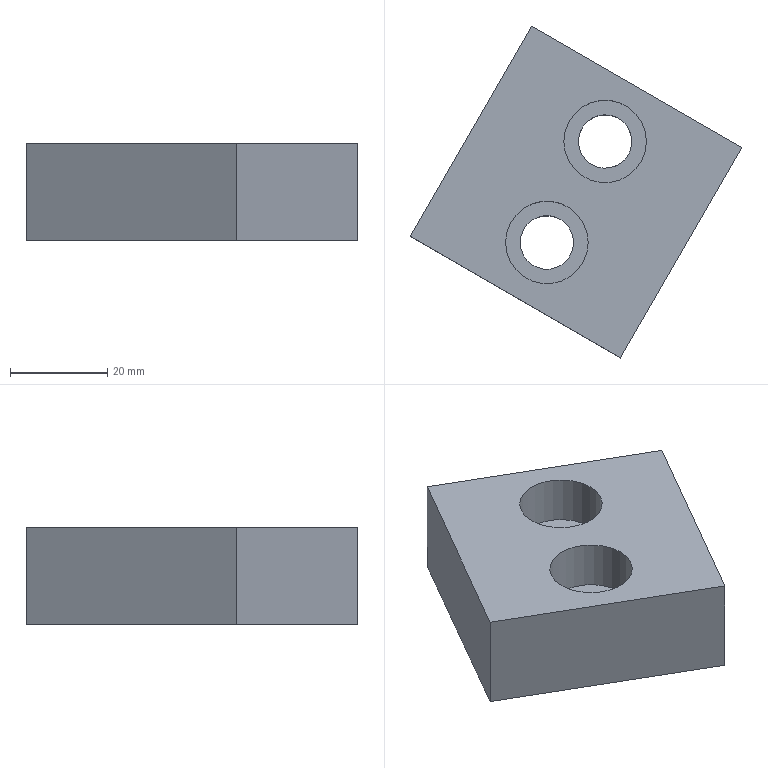Part | NX | features solid 2 | 1 solid | 12 faces | box 68.301 x 68.301 x 20 mm | volume 43560 mm3 | plane 8 | cylinder 4 | commonest cylinder face diameters 11 x2 17 x2
STEP:
#1=CARTESIAN_POINT('',(643.391,202.218,30.));
#2=VERTEX_POINT('',#1);
#3=CARTESIAN_POINT('',(668.391,245.519,30.));
#4=VERTEX_POINT('',#3);
#5=CARTESIAN_POINT('',(655.891,223.869,30.));
#6=DIRECTION('',(-0.5,-0.866,0.));
#7=VECTOR('',#6,1000.);
#8=LINE('',#5,#7);
#9=EDGE_CURVE('',#2,#4,#8,.F.);
#10=ORIENTED_EDGE('',*,*,#9,.T.);
#11=CARTESIAN_POINT('',(625.09,270.519,30.));
#12=VERTEX_POINT('',#11);
#13=CARTESIAN_POINT('',(721.058,215.112,30.));
#14=DIRECTION('',(0.866,-0.5,0.));
#15=VECTOR('',#14,1000.);
#16=LINE('',#13,#15);
#17=EDGE_CURVE('',#4,#12,#16,.F.);
#18=ORIENTED_EDGE('',*,*,#17,.T.);
#19=CARTESIAN_POINT('',(600.09,227.218,30.));
#20=VERTEX_POINT('',#19);
#21=CARTESIAN_POINT('',(625.09,270.519,30.));
#22=DIRECTION('',(0.5,0.866,0.));
#23=VECTOR('',#22,1000.);
#24=LINE('',#21,#23);
#25=EDGE_CURVE('',#12,#20,#24,.F.);
#26=ORIENTED_EDGE('',*,*,#25,.T.);
#27=CARTESIAN_POINT('',(696.058,171.811,30.));
#28=DIRECTION('',(-0.866,0.5,0.));
#29=VECTOR('',#28,1000.);
#30=LINE('',#27,#29);
#31=EDGE_CURVE('',#2,#20,#30,.T.);
#32=ORIENTED_EDGE('',*,*,#31,.F.);
#33=EDGE_LOOP('',(#10,#18,#26,#32));
#34=FACE_BOUND('',#33,.T.);
#35=CARTESIAN_POINT('',(636.74,225.976,30.));
#36=VERTEX_POINT('',#35);
#37=CARTESIAN_POINT('',(628.24,225.976,30.));
#38=DIRECTION('',(0.,0.,1.));
#39=DIRECTION('',(1.,0.,0.));
#40=AXIS2_PLACEMENT_3D('',#37,#38,#39);
#41=CIRCLE('',#40,8.5);
#42=EDGE_CURVE('',#36,#36,#41,.F.);
#43=ORIENTED_EDGE('',*,*,#42,.T.);
#44=EDGE_LOOP('',(#43));
#45=FACE_BOUND('',#44,.T.);
#46=CARTESIAN_POINT('',(648.74,246.761,30.));
#47=VERTEX_POINT('',#46);
#48=CARTESIAN_POINT('',(640.24,246.761,30.));
#49=DIRECTION('',(0.,0.,1.));
#50=DIRECTION('',(1.,0.,0.));
#51=AXIS2_PLACEMENT_3D('',#48,#49,#50);
#52=CIRCLE('',#51,8.5);
#53=EDGE_CURVE('',#47,#47,#52,.T.);
#54=ORIENTED_EDGE('',*,*,#53,.F.);
#55=EDGE_LOOP('',(#54));
#56=FACE_BOUND('',#55,.T.);
#57=CARTESIAN_POINT('',(751.058,267.073,30.));
#58=DIRECTION('',(0.,0.,1.));
#59=DIRECTION('',(-0.5,-0.866,0.));
#60=AXIS2_PLACEMENT_3D('',#57,#58,#59);
#61=PLANE('',#60);
#62=ADVANCED_FACE('',(#34,#45,#56),#61,.T.);
#63=CARTESIAN_POINT('',(622.74,225.976,10.));
#64=VERTEX_POINT('',#63);
#65=CARTESIAN_POINT('',(628.24,225.976,10.));
#66=DIRECTION('',(0.,0.,-1.));
#67=DIRECTION('',(-1.,0.,0.));
#68=AXIS2_PLACEMENT_3D('',#65,#66,#67);
#69=CIRCLE('',#68,5.5);
#70=EDGE_CURVE('',#64,#64,#69,.F.);
#71=ORIENTED_EDGE('',*,*,#70,.F.);
#72=EDGE_LOOP('',(#71));
#73=FACE_BOUND('',#72,.T.);
#74=CARTESIAN_POINT('',(622.74,225.976,20.));
#75=VERTEX_POINT('',#74);
#76=CARTESIAN_POINT('',(628.24,225.976,20.));
#77=DIRECTION('',(0.,0.,-1.));
#78=DIRECTION('',(-1.,0.,0.));
#79=AXIS2_PLACEMENT_3D('',#76,#77,#78);
#80=CIRCLE('',#79,5.5);
#81=EDGE_CURVE('',#75,#75,#80,.T.);
#82=ORIENTED_EDGE('',*,*,#81,.F.);
#83=EDGE_LOOP('',(#82));
#84=FACE_BOUND('',#83,.T.);
#85=CARTESIAN_POINT('',(628.24,225.976,30.));
#86=DIRECTION('',(0.,0.,-1.));
#87=DIRECTION('',(1.,0.,0.));
#88=AXIS2_PLACEMENT_3D('',#85,#86,#87);
#89=CYLINDRICAL_SURFACE('',#88,5.5);
#90=ADVANCED_FACE('',(#73,#84),#89,.F.);
#91=ORIENTED_EDGE('',*,*,#70,.T.);
#92=EDGE_LOOP('',(#91));
#93=FACE_BOUND('',#92,.T.);
#94=CARTESIAN_POINT('',(668.391,245.519,10.));
#95=VERTEX_POINT('',#94);
#96=CARTESIAN_POINT('',(643.391,202.218,10.));
#97=VERTEX_POINT('',#96);
#98=CARTESIAN_POINT('',(655.891,223.869,10.));
#99=DIRECTION('',(-0.5,-0.866,0.));
#100=VECTOR('',#99,1000.);
#101=LINE('',#98,#100);
#102=EDGE_CURVE('',#95,#97,#101,.T.);
#103=ORIENTED_EDGE('',*,*,#102,.T.);
#104=CARTESIAN_POINT('',(600.09,227.218,10.));
#105=VERTEX_POINT('',#104);
#106=CARTESIAN_POINT('',(696.058,171.811,10.));
#107=DIRECTION('',(0.866,-0.5,0.));
#108=VECTOR('',#107,1000.);
#109=LINE('',#106,#108);
#110=EDGE_CURVE('',#97,#105,#109,.F.);
#111=ORIENTED_EDGE('',*,*,#110,.T.);
#112=CARTESIAN_POINT('',(625.09,270.519,10.));
#113=VERTEX_POINT('',#112);
#114=CARTESIAN_POINT('',(448.115,-36.01,10.));
#115=DIRECTION('',(-0.5,-0.866,0.));
#116=VECTOR('',#115,1000.);
#117=LINE('',#114,#116);
#118=EDGE_CURVE('',#113,#105,#117,.T.);
#119=ORIENTED_EDGE('',*,*,#118,.F.);
#120=CARTESIAN_POINT('',(1116.975,-13.471,10.));
#121=DIRECTION('',(-0.866,0.5,0.));
#122=VECTOR('',#121,1000.);
#123=LINE('',#120,#122);
#124=EDGE_CURVE('',#95,#113,#123,.T.);
#125=ORIENTED_EDGE('',*,*,#124,.F.);
#126=EDGE_LOOP('',(#103,#111,#119,#125));
#127=FACE_BOUND('',#126,.T.);
#128=CARTESIAN_POINT('',(634.74,246.761,10.));
#129=VERTEX_POINT('',#128);
#130=CARTESIAN_POINT('',(640.24,246.761,10.));
#131=DIRECTION('',(0.,0.,-1.));
#132=DIRECTION('',(-1.,0.,0.));
#133=AXIS2_PLACEMENT_3D('',#130,#131,#132);
#134=CIRCLE('',#133,5.5);
#135=EDGE_CURVE('',#129,#129,#134,.F.);
#136=ORIENTED_EDGE('',*,*,#135,.T.);
#137=EDGE_LOOP('',(#136));
#138=FACE_BOUND('',#137,.T.);
#139=CARTESIAN_POINT('',(940.,-320.,10.));
#140=DIRECTION('',(0.,0.,1.));
#141=DIRECTION('',(0.,1.,0.));
#142=AXIS2_PLACEMENT_3D('',#139,#140,#141);
#143=PLANE('',#142);
#144=ADVANCED_FACE('',(#93,#127,#138),#143,.F.);
#145=CARTESIAN_POINT('',(668.391,245.519,25.));
#146=DIRECTION('',(0.,0.,-1.));
#147=VECTOR('',#146,1000.);
#148=LINE('',#145,#147);
#149=EDGE_CURVE('',#4,#95,#148,.T.);
#150=ORIENTED_EDGE('',*,*,#149,.T.);
#151=ORIENTED_EDGE('',*,*,#124,.T.);
#152=CARTESIAN_POINT('',(625.09,270.519,80.));
#153=DIRECTION('',(0.,0.,-1.));
#154=VECTOR('',#153,1000.);
#155=LINE('',#152,#154);
#156=EDGE_CURVE('',#12,#113,#155,.T.);
#157=ORIENTED_EDGE('',*,*,#156,.F.);
#158=ORIENTED_EDGE('',*,*,#17,.F.);
#159=EDGE_LOOP('',(#150,#151,#157,#158));
#160=FACE_BOUND('',#159,.T.);
#161=CARTESIAN_POINT('',(721.058,215.112,80.));
#162=DIRECTION('',(-0.5,-0.866,0.));
#163=DIRECTION('',(0.,0.,-1.));
#164=AXIS2_PLACEMENT_3D('',#161,#162,#163);
#165=PLANE('',#164);
#166=ADVANCED_FACE('',(#160),#165,.F.);
#167=CARTESIAN_POINT('',(643.391,202.218,25.));
#168=DIRECTION('',(0.,0.,-1.));
#169=VECTOR('',#168,1000.);
#170=LINE('',#167,#169);
#171=EDGE_CURVE('',#97,#2,#170,.F.);
#172=ORIENTED_EDGE('',*,*,#171,.T.);
#173=ORIENTED_EDGE('',*,*,#31,.T.);
#174=CARTESIAN_POINT('',(600.09,227.218,20.));
#175=DIRECTION('',(0.,0.,1.));
#176=VECTOR('',#175,1000.);
#177=LINE('',#174,#176);
#178=EDGE_CURVE('',#20,#105,#177,.F.);
#179=ORIENTED_EDGE('',*,*,#178,.T.);
#180=ORIENTED_EDGE('',*,*,#110,.F.);
#181=EDGE_LOOP('',(#172,#173,#179,#180));
#182=FACE_BOUND('',#181,.T.);
#183=CARTESIAN_POINT('',(696.058,171.811,80.));
#184=DIRECTION('',(-0.5,-0.866,0.));
#185=DIRECTION('',(0.,0.,-1.));
#186=AXIS2_PLACEMENT_3D('',#183,#184,#185);
#187=PLANE('',#186);
#188=ADVANCED_FACE('',(#182),#187,.T.);
#189=ORIENTED_EDGE('',*,*,#118,.T.);
#190=ORIENTED_EDGE('',*,*,#178,.F.);
#191=ORIENTED_EDGE('',*,*,#25,.F.);
#192=ORIENTED_EDGE('',*,*,#156,.T.);
#193=EDGE_LOOP('',(#189,#190,#191,#192));
#194=FACE_BOUND('',#193,.T.);
#195=CARTESIAN_POINT('',(625.09,270.519,20.));
#196=DIRECTION('',(-0.866,0.5,0.));
#197=DIRECTION('',(0.5,0.866,0.));
#198=AXIS2_PLACEMENT_3D('',#195,#196,#197);
#199=PLANE('',#198);
#200=ADVANCED_FACE('',(#194),#199,.T.);
#201=ORIENTED_EDGE('',*,*,#171,.F.);
#202=ORIENTED_EDGE('',*,*,#102,.F.);
#203=ORIENTED_EDGE('',*,*,#149,.F.);
#204=ORIENTED_EDGE('',*,*,#9,.F.);
#205=EDGE_LOOP('',(#201,#202,#203,#204));
#206=FACE_BOUND('',#205,.T.);
#207=CARTESIAN_POINT('',(655.891,223.869,25.));
#208=DIRECTION('',(0.866,-0.5,0.));
#209=DIRECTION('',(-0.5,-0.866,0.));
#210=AXIS2_PLACEMENT_3D('',#207,#208,#209);
#211=PLANE('',#210);
#212=ADVANCED_FACE('',(#206),#211,.T.);
#213=CARTESIAN_POINT('',(637.49,251.524,20.));
#214=VERTEX_POINT('',#213);
#215=CARTESIAN_POINT('',(640.24,246.761,20.));
#216=DIRECTION('',(0.,0.,1.));
#217=DIRECTION('',(-0.5,0.866,0.));
#218=AXIS2_PLACEMENT_3D('',#215,#216,#217);
#219=CIRCLE('',#218,5.5);
#220=EDGE_CURVE('',#214,#214,#219,.T.);
#221=ORIENTED_EDGE('',*,*,#220,.T.);
#222=EDGE_LOOP('',(#221));
#223=FACE_BOUND('',#222,.T.);
#224=ORIENTED_EDGE('',*,*,#135,.F.);
#225=EDGE_LOOP('',(#224));
#226=FACE_BOUND('',#225,.T.);
#227=CARTESIAN_POINT('',(640.24,246.761,30.));
#228=DIRECTION('',(0.,0.,-1.));
#229=DIRECTION('',(0.5,-0.866,0.));
#230=AXIS2_PLACEMENT_3D('',#227,#228,#229);
#231=CYLINDRICAL_SURFACE('',#230,5.5);
#232=ADVANCED_FACE('',(#223,#226),#231,.F.);
#233=CARTESIAN_POINT('',(619.74,225.976,20.));
#234=VERTEX_POINT('',#233);
#235=CARTESIAN_POINT('',(628.24,225.976,20.));
#236=DIRECTION('',(0.,0.,-1.));
#237=DIRECTION('',(-1.,0.,0.));
#238=AXIS2_PLACEMENT_3D('',#235,#236,#237);
#239=CIRCLE('',#238,8.5);
#240=EDGE_CURVE('',#234,#234,#239,.T.);
#241=ORIENTED_EDGE('',*,*,#240,.T.);
#242=EDGE_LOOP('',(#241));
#243=FACE_BOUND('',#242,.T.);
#244=ORIENTED_EDGE('',*,*,#42,.F.);
#245=EDGE_LOOP('',(#244));
#246=FACE_BOUND('',#245,.T.);
#247=CARTESIAN_POINT('',(628.24,225.976,35.));
#248=DIRECTION('',(0.,0.,-1.));
#249=DIRECTION('',(-1.,0.,0.));
#250=AXIS2_PLACEMENT_3D('',#247,#248,#249);
#251=CYLINDRICAL_SURFACE('',#250,8.5);
#252=ADVANCED_FACE('',(#243,#246),#251,.F.);
#253=ORIENTED_EDGE('',*,*,#240,.F.);
#254=EDGE_LOOP('',(#253));
#255=FACE_BOUND('',#254,.T.);
#256=ORIENTED_EDGE('',*,*,#81,.T.);
#257=EDGE_LOOP('',(#256));
#258=FACE_BOUND('',#257,.T.);
#259=CARTESIAN_POINT('',(628.946,225.569,20.));
#260=DIRECTION('',(0.,0.,1.));
#261=DIRECTION('',(1.,0.,0.));
#262=AXIS2_PLACEMENT_3D('',#259,#260,#261);
#263=PLANE('',#262);
#264=ADVANCED_FACE('',(#255,#258),#263,.T.);
#265=CARTESIAN_POINT('',(631.74,246.761,20.));
#266=VERTEX_POINT('',#265);
#267=CARTESIAN_POINT('',(640.24,246.761,20.));
#268=DIRECTION('',(0.,0.,-1.));
#269=DIRECTION('',(-1.,0.,0.));
#270=AXIS2_PLACEMENT_3D('',#267,#268,#269);
#271=CIRCLE('',#270,8.5);
#272=EDGE_CURVE('',#266,#266,#271,.F.);
#273=ORIENTED_EDGE('',*,*,#272,.F.);
#274=EDGE_LOOP('',(#273));
#275=FACE_BOUND('',#274,.T.);
#276=ORIENTED_EDGE('',*,*,#53,.T.);
#277=EDGE_LOOP('',(#276));
#278=FACE_BOUND('',#277,.T.);
#279=CARTESIAN_POINT('',(640.24,246.761,35.));
#280=DIRECTION('',(0.,0.,-1.));
#281=DIRECTION('',(-1.,0.,0.));
#282=AXIS2_PLACEMENT_3D('',#279,#280,#281);
#283=CYLINDRICAL_SURFACE('',#282,8.5);
#284=ADVANCED_FACE('',(#275,#278),#283,.F.);
#285=ORIENTED_EDGE('',*,*,#272,.T.);
#286=EDGE_LOOP('',(#285));
#287=FACE_BOUND('',#286,.T.);
#288=ORIENTED_EDGE('',*,*,#220,.F.);
#289=EDGE_LOOP('',(#288));
#290=FACE_BOUND('',#289,.T.);
#291=CARTESIAN_POINT('',(640.946,246.354,20.));
#292=DIRECTION('',(0.,0.,-1.));
#293=DIRECTION('',(-1.,0.,0.));
#294=AXIS2_PLACEMENT_3D('',#291,#292,#293);
#295=PLANE('',#294);
#296=ADVANCED_FACE('',(#287,#290),#295,.F.);
#297=CLOSED_SHELL('',(#62,#90,#144,#166,#188,#200,#212,#232,#252,#264,#284,#296));
#298=MANIFOLD_SOLID_BREP('',#297);
#299=(LENGTH_UNIT()NAMED_UNIT(*)SI_UNIT(.MILLI.,.METRE.));
#300=UNCERTAINTY_MEASURE_WITH_UNIT(LENGTH_MEASURE(0.00001),#299,'','');
#301=(NAMED_UNIT(*)PLANE_ANGLE_UNIT()SI_UNIT($,.RADIAN.));
#302=(NAMED_UNIT(*)SI_UNIT($,.STERADIAN.)SOLID_ANGLE_UNIT());
#303=(GEOMETRIC_REPRESENTATION_CONTEXT(3)GLOBAL_UNCERTAINTY_ASSIGNED_CONTEXT((#300))GLOBAL_UNIT_ASSIGNED_CONTEXT((#299,#301,#302))REPRESENTATION_CONTEXT('',''));
#304=ADVANCED_BREP_SHAPE_REPRESENTATION('',(#298),#303);